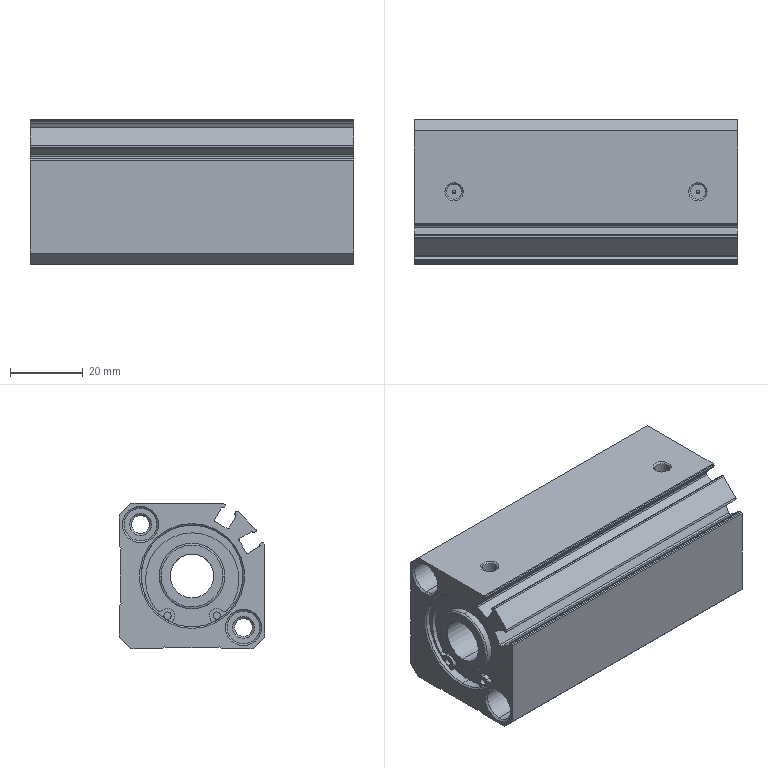Part | STEP file | ACQJ25x50-10S-01-cc | 1 solid | 163 faces | box 89 x 40 x 40 mm | volume 88799 mm3 | cylinder 79 | plane 56 | cone 24 | spline 4 | commonest cylinder face diameters 0.8 x11 2 x8 9 x8 1 x7 0.4 x6 2.4 x6